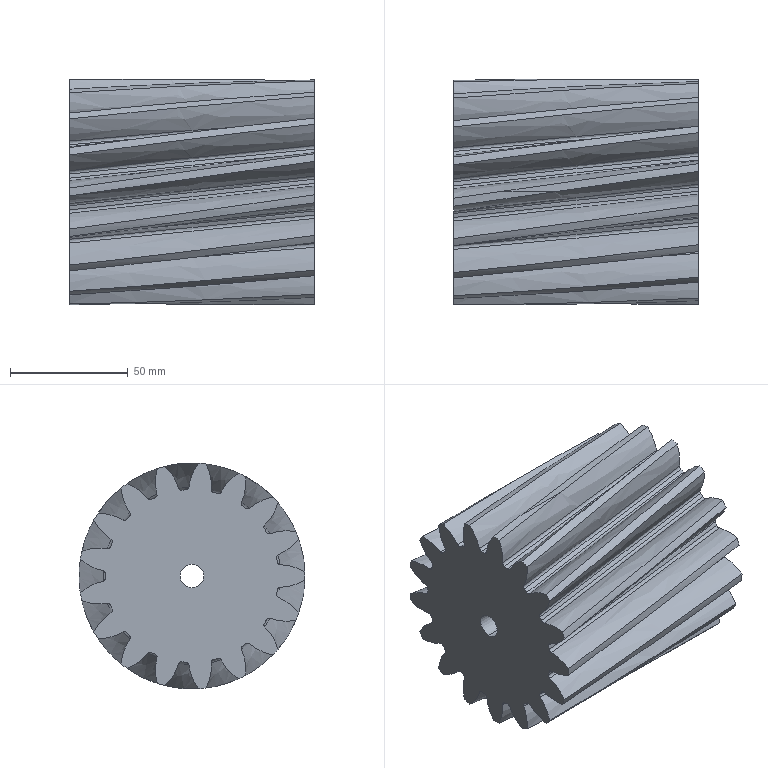Part | SolidWorks | features Boss 3, CirPattern 3, Cut 2, Helix 2, SweepCut 2, Revolution 1 | 1 solid | 107 faces | box 104 x 95.86 x 95.86 mm | volume 585543 mm3 | spline 85 | cylinder 20 | plane 2 | commonest cylinder face diameters 95.86 x18 10 x2